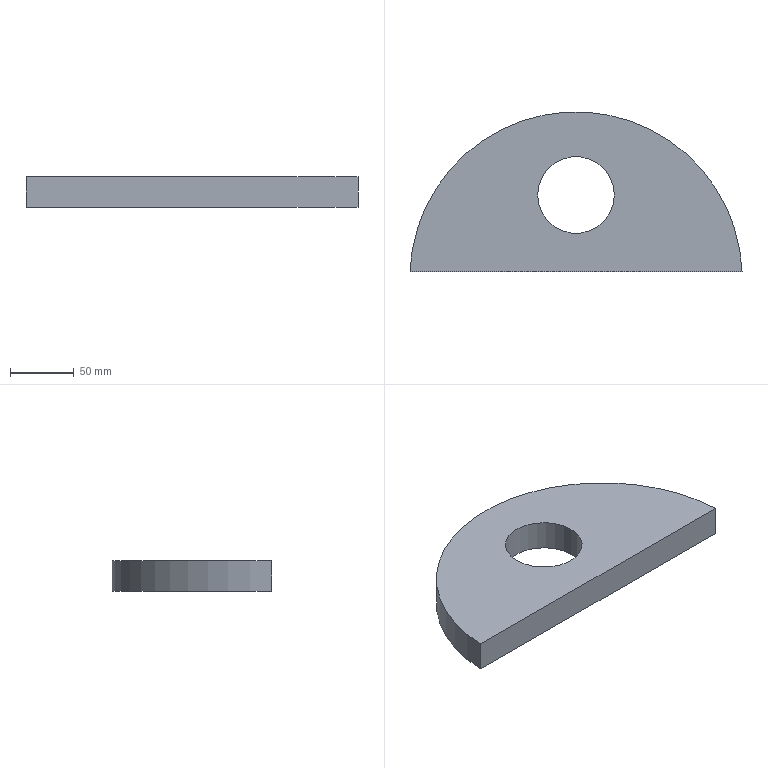Part | SolidWorks | features Extrusion 1 | 1 solid | 6 faces | box 259.808 x 125 x 24 mm | volume 538064 mm3 | cylinder 3 | plane 3 | commonest cylinder face diameters 60 x2 260 x1
STEP:
#1=CARTESIAN_POINT('',(-30.,65.,12.));
#2=VERTEX_POINT('',#1);
#3=CARTESIAN_POINT('',(30.,65.,12.));
#4=VERTEX_POINT('',#3);
#5=CARTESIAN_POINT('',(0.,65.,12.));
#6=DIRECTION('',(0.,0.,1.));
#7=DIRECTION('',(1.,0.,0.));
#8=AXIS2_PLACEMENT_3D('',#5,#6,#7);
#9=CIRCLE('',#8,30.);
#10=EDGE_CURVE('',#2,#4,#9,.T.);
#11=ORIENTED_EDGE('',*,*,#10,.T.);
#12=CARTESIAN_POINT('',(30.,65.,-12.));
#13=VERTEX_POINT('',#12);
#14=CARTESIAN_POINT('',(30.,65.,12.));
#15=DIRECTION('',(0.,0.,-1.));
#16=VECTOR('',#15,1000.);
#17=LINE('',#14,#16);
#18=EDGE_CURVE('',#4,#13,#17,.T.);
#19=ORIENTED_EDGE('',*,*,#18,.T.);
#20=CARTESIAN_POINT('',(-30.,65.,-12.));
#21=VERTEX_POINT('',#20);
#22=CARTESIAN_POINT('',(0.,65.,-12.));
#23=DIRECTION('',(0.,0.,1.));
#24=DIRECTION('',(1.,0.,0.));
#25=AXIS2_PLACEMENT_3D('',#22,#23,#24);
#26=CIRCLE('',#25,30.);
#27=EDGE_CURVE('',#21,#13,#26,.T.);
#28=ORIENTED_EDGE('',*,*,#27,.F.);
#29=CARTESIAN_POINT('',(-30.,65.,12.));
#30=DIRECTION('',(0.,0.,-1.));
#31=VECTOR('',#30,1000.);
#32=LINE('',#29,#31);
#33=EDGE_CURVE('',#2,#21,#32,.T.);
#34=ORIENTED_EDGE('',*,*,#33,.F.);
#35=EDGE_LOOP('',(#11,#19,#28,#34));
#36=FACE_OUTER_BOUND('',#35,.T.);
#37=CARTESIAN_POINT('',(0.,65.,12.));
#38=DIRECTION('',(0.,0.,-1.));
#39=DIRECTION('',(-1.,0.,0.));
#40=AXIS2_PLACEMENT_3D('',#37,#38,#39);
#41=CYLINDRICAL_SURFACE('',#40,30.);
#42=ADVANCED_FACE('',(#36),#41,.F.);
#43=CARTESIAN_POINT('',(129.904,5.,12.));
#44=VERTEX_POINT('',#43);
#45=CARTESIAN_POINT('',(-129.904,5.,12.));
#46=VERTEX_POINT('',#45);
#47=CARTESIAN_POINT('',(0.,0.,12.));
#48=DIRECTION('',(0.,0.,1.));
#49=DIRECTION('',(1.,0.,0.));
#50=AXIS2_PLACEMENT_3D('',#47,#48,#49);
#51=CIRCLE('',#50,130.);
#52=EDGE_CURVE('',#44,#46,#51,.T.);
#53=ORIENTED_EDGE('',*,*,#52,.T.);
#54=CARTESIAN_POINT('',(-129.904,5.,12.));
#55=DIRECTION('',(1.,0.,0.));
#56=VECTOR('',#55,1000.);
#57=LINE('',#54,#56);
#58=EDGE_CURVE('',#46,#44,#57,.T.);
#59=ORIENTED_EDGE('',*,*,#58,.T.);
#60=EDGE_LOOP('',(#53,#59));
#61=FACE_OUTER_BOUND('',#60,.T.);
#62=ORIENTED_EDGE('',*,*,#10,.F.);
#63=CARTESIAN_POINT('',(0.,65.,12.));
#64=DIRECTION('',(0.,0.,1.));
#65=DIRECTION('',(1.,0.,0.));
#66=AXIS2_PLACEMENT_3D('',#63,#64,#65);
#67=CIRCLE('',#66,30.);
#68=EDGE_CURVE('',#4,#2,#67,.T.);
#69=ORIENTED_EDGE('',*,*,#68,.F.);
#70=EDGE_LOOP('',(#62,#69));
#71=FACE_BOUND('',#70,.T.);
#72=CARTESIAN_POINT('',(0.,0.,12.));
#73=DIRECTION('',(0.,0.,1.));
#74=DIRECTION('',(1.,0.,0.));
#75=AXIS2_PLACEMENT_3D('',#72,#73,#74);
#76=PLANE('',#75);
#77=ADVANCED_FACE('',(#61,#71),#76,.T.);
#78=CARTESIAN_POINT('',(129.904,5.,-12.));
#79=VERTEX_POINT('',#78);
#80=CARTESIAN_POINT('',(-129.904,5.,-12.));
#81=VERTEX_POINT('',#80);
#82=CARTESIAN_POINT('',(0.,0.,-12.));
#83=DIRECTION('',(0.,0.,1.));
#84=DIRECTION('',(1.,0.,0.));
#85=AXIS2_PLACEMENT_3D('',#82,#83,#84);
#86=CIRCLE('',#85,130.);
#87=EDGE_CURVE('',#79,#81,#86,.T.);
#88=ORIENTED_EDGE('',*,*,#87,.F.);
#89=CARTESIAN_POINT('',(-129.904,5.,-12.));
#90=DIRECTION('',(1.,0.,0.));
#91=VECTOR('',#90,1000.);
#92=LINE('',#89,#91);
#93=EDGE_CURVE('',#81,#79,#92,.T.);
#94=ORIENTED_EDGE('',*,*,#93,.F.);
#95=EDGE_LOOP('',(#88,#94));
#96=FACE_OUTER_BOUND('',#95,.T.);
#97=ORIENTED_EDGE('',*,*,#27,.T.);
#98=CARTESIAN_POINT('',(0.,65.,-12.));
#99=DIRECTION('',(0.,0.,1.));
#100=DIRECTION('',(1.,0.,0.));
#101=AXIS2_PLACEMENT_3D('',#98,#99,#100);
#102=CIRCLE('',#101,30.);
#103=EDGE_CURVE('',#13,#21,#102,.T.);
#104=ORIENTED_EDGE('',*,*,#103,.T.);
#105=EDGE_LOOP('',(#97,#104));
#106=FACE_BOUND('',#105,.T.);
#107=CARTESIAN_POINT('',(0.,0.,-12.));
#108=DIRECTION('',(0.,0.,1.));
#109=DIRECTION('',(1.,0.,0.));
#110=AXIS2_PLACEMENT_3D('',#107,#108,#109);
#111=PLANE('',#110);
#112=ADVANCED_FACE('',(#96,#106),#111,.F.);
#113=ORIENTED_EDGE('',*,*,#87,.T.);
#114=CARTESIAN_POINT('',(-129.904,5.,12.));
#115=DIRECTION('',(0.,0.,-1.));
#116=VECTOR('',#115,1000.);
#117=LINE('',#114,#116);
#118=EDGE_CURVE('',#46,#81,#117,.T.);
#119=ORIENTED_EDGE('',*,*,#118,.F.);
#120=ORIENTED_EDGE('',*,*,#52,.F.);
#121=CARTESIAN_POINT('',(129.904,5.,12.));
#122=DIRECTION('',(0.,0.,-1.));
#123=VECTOR('',#122,1000.);
#124=LINE('',#121,#123);
#125=EDGE_CURVE('',#44,#79,#124,.T.);
#126=ORIENTED_EDGE('',*,*,#125,.T.);
#127=EDGE_LOOP('',(#113,#119,#120,#126));
#128=FACE_OUTER_BOUND('',#127,.T.);
#129=CARTESIAN_POINT('',(0.,0.,12.));
#130=DIRECTION('',(0.,0.,-1.));
#131=DIRECTION('',(-1.,0.,0.));
#132=AXIS2_PLACEMENT_3D('',#129,#130,#131);
#133=CYLINDRICAL_SURFACE('',#132,130.);
#134=ADVANCED_FACE('',(#128),#133,.T.);
#135=ORIENTED_EDGE('',*,*,#93,.T.);
#136=ORIENTED_EDGE('',*,*,#125,.F.);
#137=ORIENTED_EDGE('',*,*,#58,.F.);
#138=ORIENTED_EDGE('',*,*,#118,.T.);
#139=EDGE_LOOP('',(#135,#136,#137,#138));
#140=FACE_OUTER_BOUND('',#139,.T.);
#141=CARTESIAN_POINT('',(-129.904,5.,12.));
#142=DIRECTION('',(0.,1.,0.));
#143=DIRECTION('',(0.,0.,1.));
#144=AXIS2_PLACEMENT_3D('',#141,#142,#143);
#145=PLANE('',#144);
#146=ADVANCED_FACE('',(#140),#145,.F.);
#147=ORIENTED_EDGE('',*,*,#18,.F.);
#148=ORIENTED_EDGE('',*,*,#68,.T.);
#149=ORIENTED_EDGE('',*,*,#33,.T.);
#150=ORIENTED_EDGE('',*,*,#103,.F.);
#151=EDGE_LOOP('',(#147,#148,#149,#150));
#152=FACE_OUTER_BOUND('',#151,.T.);
#153=CARTESIAN_POINT('',(0.,65.,12.));
#154=DIRECTION('',(0.,0.,-1.));
#155=DIRECTION('',(-1.,0.,0.));
#156=AXIS2_PLACEMENT_3D('',#153,#154,#155);
#157=CYLINDRICAL_SURFACE('',#156,30.);
#158=ADVANCED_FACE('',(#152),#157,.F.);
#159=CLOSED_SHELL('',(#42,#77,#112,#134,#146,#158));
#160=MANIFOLD_SOLID_BREP('',#159);
#161=CARTESIAN_POINT('',(0.,0.,0.));
#162=DIRECTION('',(0.,0.,1.));
#163=DIRECTION('',(1.,0.,0.));
#164=AXIS2_PLACEMENT_3D('',#161,#162,#163);
#165=(LENGTH_UNIT()NAMED_UNIT(*)SI_UNIT(.MILLI.,.METRE.));
#166=UNCERTAINTY_MEASURE_WITH_UNIT(LENGTH_MEASURE(0.00001),#165,'','');
#167=(NAMED_UNIT(*)PLANE_ANGLE_UNIT()SI_UNIT($,.RADIAN.));
#168=(NAMED_UNIT(*)SI_UNIT($,.STERADIAN.)SOLID_ANGLE_UNIT());
#169=(GEOMETRIC_REPRESENTATION_CONTEXT(3)GLOBAL_UNCERTAINTY_ASSIGNED_CONTEXT((#166))GLOBAL_UNIT_ASSIGNED_CONTEXT((#165,#167,#168))REPRESENTATION_CONTEXT('',''));
#170=ADVANCED_BREP_SHAPE_REPRESENTATION('',(#160,#164),#169);